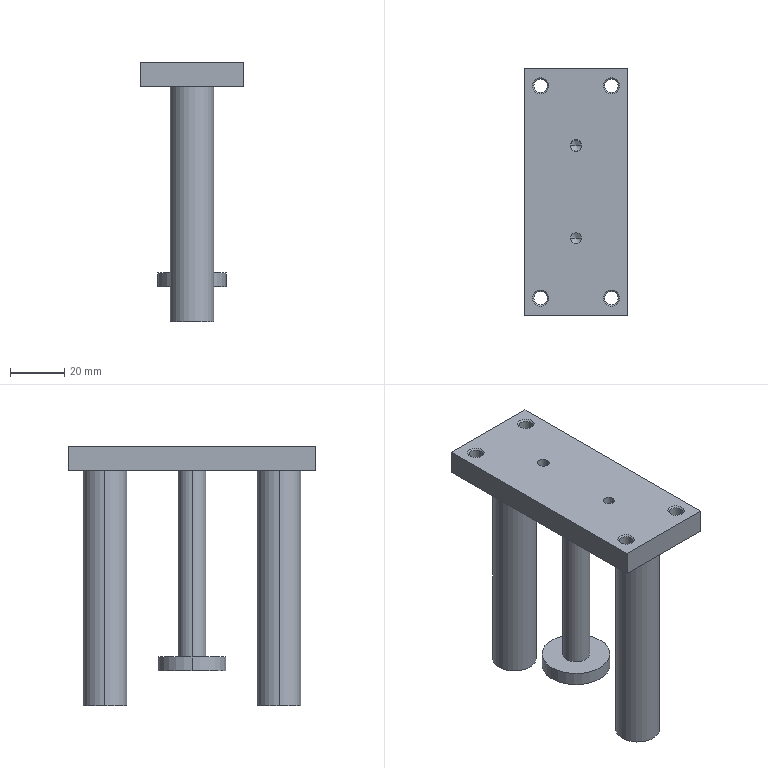Part | SolidWorks | features BaseBody 1 | 1 solid | 56 faces | box 38 x 91 x 95.5 mm | volume 72871 mm3 | cylinder 22 | cone 20 | plane 14 | commonest cylinder face diameters 4.917 x8 4 x6 16 x4 10 x2 25 x2
STEP:
#1=CARTESIAN_POINT('',(-8.,32.,7.));
#2=VERTEX_POINT('',#1);
#3=CARTESIAN_POINT('',(8.,32.,7.));
#4=VERTEX_POINT('',#3);
#5=CARTESIAN_POINT('',(0.,32.,7.));
#6=DIRECTION('',(0.,0.,-1.));
#7=DIRECTION('',(-1.,0.,0.));
#8=AXIS2_PLACEMENT_3D('',#5,#6,#7);
#9=CIRCLE('',#8,8.);
#10=EDGE_CURVE('',#2,#4,#9,.T.);
#11=ORIENTED_EDGE('',*,*,#10,.T.);
#12=CARTESIAN_POINT('',(8.,32.,-79.5));
#13=VERTEX_POINT('',#12);
#14=CARTESIAN_POINT('',(8.,32.,-87.5));
#15=DIRECTION('',(0.,0.,-1.));
#16=VECTOR('',#15,1000.);
#17=LINE('',#14,#16);
#18=EDGE_CURVE('',#4,#13,#17,.T.);
#19=ORIENTED_EDGE('',*,*,#18,.T.);
#20=CARTESIAN_POINT('',(-8.,32.,-79.5));
#21=VERTEX_POINT('',#20);
#22=CARTESIAN_POINT('',(0.,32.,-79.5));
#23=DIRECTION('',(0.,0.,1.));
#24=DIRECTION('',(-1.,0.,0.));
#25=AXIS2_PLACEMENT_3D('',#22,#23,#24);
#26=CIRCLE('',#25,8.);
#27=EDGE_CURVE('',#13,#21,#26,.T.);
#28=ORIENTED_EDGE('',*,*,#27,.T.);
#29=CARTESIAN_POINT('',(-8.,32.,-87.5));
#30=DIRECTION('',(0.,0.,-1.));
#31=VECTOR('',#30,1000.);
#32=LINE('',#29,#31);
#33=EDGE_CURVE('',#2,#21,#32,.T.);
#34=ORIENTED_EDGE('',*,*,#33,.F.);
#35=EDGE_LOOP('',(#11,#19,#28,#34));
#36=FACE_OUTER_BOUND('',#35,.T.);
#37=CARTESIAN_POINT('',(0.,32.,-87.5));
#38=DIRECTION('',(0.,0.,-1.));
#39=DIRECTION('',(-1.,0.,0.));
#40=AXIS2_PLACEMENT_3D('',#37,#38,#39);
#41=CYLINDRICAL_SURFACE('',#40,8.);
#42=ADVANCED_FACE('',(#36),#41,.T.);
#43=CARTESIAN_POINT('',(-8.,-32.,7.));
#44=VERTEX_POINT('',#43);
#45=CARTESIAN_POINT('',(8.,-32.,7.));
#46=VERTEX_POINT('',#45);
#47=CARTESIAN_POINT('',(0.,-32.,7.));
#48=DIRECTION('',(0.,0.,-1.));
#49=DIRECTION('',(-1.,0.,0.));
#50=AXIS2_PLACEMENT_3D('',#47,#48,#49);
#51=CIRCLE('',#50,8.);
#52=EDGE_CURVE('',#44,#46,#51,.T.);
#53=ORIENTED_EDGE('',*,*,#52,.T.);
#54=CARTESIAN_POINT('',(8.,-32.,-79.5));
#55=VERTEX_POINT('',#54);
#56=CARTESIAN_POINT('',(8.,-32.,-87.5));
#57=DIRECTION('',(0.,0.,-1.));
#58=VECTOR('',#57,1000.);
#59=LINE('',#56,#58);
#60=EDGE_CURVE('',#46,#55,#59,.T.);
#61=ORIENTED_EDGE('',*,*,#60,.T.);
#62=CARTESIAN_POINT('',(-8.,-32.,-79.5));
#63=VERTEX_POINT('',#62);
#64=CARTESIAN_POINT('',(0.,-32.,-79.5));
#65=DIRECTION('',(0.,0.,1.));
#66=DIRECTION('',(-1.,0.,0.));
#67=AXIS2_PLACEMENT_3D('',#64,#65,#66);
#68=CIRCLE('',#67,8.);
#69=EDGE_CURVE('',#55,#63,#68,.T.);
#70=ORIENTED_EDGE('',*,*,#69,.T.);
#71=CARTESIAN_POINT('',(-8.,-32.,-87.5));
#72=DIRECTION('',(0.,0.,-1.));
#73=VECTOR('',#72,1000.);
#74=LINE('',#71,#73);
#75=EDGE_CURVE('',#44,#63,#74,.T.);
#76=ORIENTED_EDGE('',*,*,#75,.F.);
#77=EDGE_LOOP('',(#53,#61,#70,#76));
#78=FACE_OUTER_BOUND('',#77,.T.);
#79=CARTESIAN_POINT('',(0.,-32.,-87.5));
#80=DIRECTION('',(0.,0.,-1.));
#81=DIRECTION('',(-1.,0.,0.));
#82=AXIS2_PLACEMENT_3D('',#79,#80,#81);
#83=CYLINDRICAL_SURFACE('',#82,8.);
#84=ADVANCED_FACE('',(#78),#83,.T.);
#85=CARTESIAN_POINT('',(5.,0.,-61.5));
#86=VERTEX_POINT('',#85);
#87=CARTESIAN_POINT('',(-5.,0.,-61.5));
#88=VERTEX_POINT('',#87);
#89=CARTESIAN_POINT('',(0.,0.,-61.5));
#90=DIRECTION('',(0.,0.,1.));
#91=DIRECTION('',(1.,0.,0.));
#92=AXIS2_PLACEMENT_3D('',#89,#90,#91);
#93=CIRCLE('',#92,5.);
#94=EDGE_CURVE('',#86,#88,#93,.T.);
#95=ORIENTED_EDGE('',*,*,#94,.T.);
#96=CARTESIAN_POINT('',(-5.,0.,7.));
#97=VERTEX_POINT('',#96);
#98=CARTESIAN_POINT('',(-5.,0.,-66.5));
#99=DIRECTION('',(0.,0.,1.));
#100=VECTOR('',#99,1000.);
#101=LINE('',#98,#100);
#102=EDGE_CURVE('',#88,#97,#101,.T.);
#103=ORIENTED_EDGE('',*,*,#102,.T.);
#104=CARTESIAN_POINT('',(5.,0.,7.));
#105=VERTEX_POINT('',#104);
#106=CARTESIAN_POINT('',(0.,0.,7.));
#107=DIRECTION('',(0.,0.,-1.));
#108=DIRECTION('',(1.,0.,0.));
#109=AXIS2_PLACEMENT_3D('',#106,#107,#108);
#110=CIRCLE('',#109,5.);
#111=EDGE_CURVE('',#97,#105,#110,.T.);
#112=ORIENTED_EDGE('',*,*,#111,.T.);
#113=CARTESIAN_POINT('',(5.,0.,-66.5));
#114=DIRECTION('',(0.,0.,1.));
#115=VECTOR('',#114,1000.);
#116=LINE('',#113,#115);
#117=EDGE_CURVE('',#86,#105,#116,.T.);
#118=ORIENTED_EDGE('',*,*,#117,.F.);
#119=EDGE_LOOP('',(#95,#103,#112,#118));
#120=FACE_OUTER_BOUND('',#119,.T.);
#121=CARTESIAN_POINT('',(0.,0.,-66.5));
#122=DIRECTION('',(0.,0.,1.));
#123=DIRECTION('',(1.,0.,0.));
#124=AXIS2_PLACEMENT_3D('',#121,#122,#123);
#125=CYLINDRICAL_SURFACE('',#124,5.);
#126=ADVANCED_FACE('',(#120),#125,.T.);
#127=CARTESIAN_POINT('',(15.459,-39.,7.542));
#128=VERTEX_POINT('',#127);
#129=CARTESIAN_POINT('',(10.541,-39.,7.542));
#130=VERTEX_POINT('',#129);
#131=CARTESIAN_POINT('',(13.,-39.,7.542));
#132=DIRECTION('',(0.,0.,-1.));
#133=DIRECTION('',(-1.,0.,0.));
#134=AXIS2_PLACEMENT_3D('',#131,#132,#133);
#135=CIRCLE('',#134,2.459);
#136=EDGE_CURVE('',#128,#130,#135,.T.);
#137=ORIENTED_EDGE('',*,*,#136,.F.);
#138=CARTESIAN_POINT('',(16.,-39.,7.));
#139=VERTEX_POINT('',#138);
#140=CARTESIAN_POINT('',(16.,-39.,7.));
#141=DIRECTION('',(0.7071,0.,-0.7071));
#142=VECTOR('',#141,1000.);
#143=LINE('',#140,#142);
#144=EDGE_CURVE('',#128,#139,#143,.T.);
#145=ORIENTED_EDGE('',*,*,#144,.T.);
#146=CARTESIAN_POINT('',(10.,-39.,7.));
#147=VERTEX_POINT('',#146);
#148=CARTESIAN_POINT('',(13.,-39.,7.));
#149=DIRECTION('',(0.,0.,-1.));
#150=DIRECTION('',(-1.,0.,0.));
#151=AXIS2_PLACEMENT_3D('',#148,#149,#150);
#152=CIRCLE('',#151,3.);
#153=EDGE_CURVE('',#139,#147,#152,.T.);
#154=ORIENTED_EDGE('',*,*,#153,.T.);
#155=CARTESIAN_POINT('',(10.,-39.,7.));
#156=DIRECTION('',(-0.7071,0.,-0.7071));
#157=VECTOR('',#156,1000.);
#158=LINE('',#155,#157);
#159=EDGE_CURVE('',#130,#147,#158,.T.);
#160=ORIENTED_EDGE('',*,*,#159,.F.);
#161=EDGE_LOOP('',(#137,#145,#154,#160));
#162=FACE_OUTER_BOUND('',#161,.T.);
#163=CARTESIAN_POINT('',(13.,-39.,7.));
#164=DIRECTION('',(0.,0.,-1.));
#165=DIRECTION('',(-1.,0.,0.));
#166=AXIS2_PLACEMENT_3D('',#163,#164,#165);
#167=CONICAL_SURFACE('',#166,3.,0.7854);
#168=ADVANCED_FACE('',(#162),#167,.F.);
#169=CARTESIAN_POINT('',(-10.541,-39.,7.542));
#170=VERTEX_POINT('',#169);
#171=CARTESIAN_POINT('',(-15.459,-39.,7.542));
#172=VERTEX_POINT('',#171);
#173=CARTESIAN_POINT('',(-13.,-39.,7.542));
#174=DIRECTION('',(0.,0.,-1.));
#175=DIRECTION('',(-1.,0.,0.));
#176=AXIS2_PLACEMENT_3D('',#173,#174,#175);
#177=CIRCLE('',#176,2.459);
#178=EDGE_CURVE('',#170,#172,#177,.T.);
#179=ORIENTED_EDGE('',*,*,#178,.F.);
#180=CARTESIAN_POINT('',(-10.,-39.,7.));
#181=VERTEX_POINT('',#180);
#182=CARTESIAN_POINT('',(-10.,-39.,7.));
#183=DIRECTION('',(0.7071,0.,-0.7071));
#184=VECTOR('',#183,1000.);
#185=LINE('',#182,#184);
#186=EDGE_CURVE('',#170,#181,#185,.T.);
#187=ORIENTED_EDGE('',*,*,#186,.T.);
#188=CARTESIAN_POINT('',(-16.,-39.,7.));
#189=VERTEX_POINT('',#188);
#190=CARTESIAN_POINT('',(-13.,-39.,7.));
#191=DIRECTION('',(0.,0.,-1.));
#192=DIRECTION('',(-1.,0.,0.));
#193=AXIS2_PLACEMENT_3D('',#190,#191,#192);
#194=CIRCLE('',#193,3.);
#195=EDGE_CURVE('',#181,#189,#194,.T.);
#196=ORIENTED_EDGE('',*,*,#195,.T.);
#197=CARTESIAN_POINT('',(-16.,-39.,7.));
#198=DIRECTION('',(-0.7071,0.,-0.7071));
#199=VECTOR('',#198,1000.);
#200=LINE('',#197,#199);
#201=EDGE_CURVE('',#172,#189,#200,.T.);
#202=ORIENTED_EDGE('',*,*,#201,.F.);
#203=EDGE_LOOP('',(#179,#187,#196,#202));
#204=FACE_OUTER_BOUND('',#203,.T.);
#205=CARTESIAN_POINT('',(-13.,-39.,7.));
#206=DIRECTION('',(0.,0.,-1.));
#207=DIRECTION('',(-1.,0.,0.));
#208=AXIS2_PLACEMENT_3D('',#205,#206,#207);
#209=CONICAL_SURFACE('',#208,3.,0.7854);
#210=ADVANCED_FACE('',(#204),#209,.F.);
#211=CARTESIAN_POINT('',(15.459,39.,7.542));
#212=VERTEX_POINT('',#211);
#213=CARTESIAN_POINT('',(10.541,39.,7.542));
#214=VERTEX_POINT('',#213);
#215=CARTESIAN_POINT('',(13.,39.,7.542));
#216=DIRECTION('',(0.,0.,-1.));
#217=DIRECTION('',(-1.,0.,0.));
#218=AXIS2_PLACEMENT_3D('',#215,#216,#217);
#219=CIRCLE('',#218,2.459);
#220=EDGE_CURVE('',#212,#214,#219,.T.);
#221=ORIENTED_EDGE('',*,*,#220,.F.);
#222=CARTESIAN_POINT('',(16.,39.,7.));
#223=VERTEX_POINT('',#222);
#224=CARTESIAN_POINT('',(16.,39.,7.));
#225=DIRECTION('',(0.7071,0.,-0.7071));
#226=VECTOR('',#225,1000.);
#227=LINE('',#224,#226);
#228=EDGE_CURVE('',#212,#223,#227,.T.);
#229=ORIENTED_EDGE('',*,*,#228,.T.);
#230=CARTESIAN_POINT('',(10.,39.,7.));
#231=VERTEX_POINT('',#230);
#232=CARTESIAN_POINT('',(13.,39.,7.));
#233=DIRECTION('',(0.,0.,-1.));
#234=DIRECTION('',(-1.,0.,0.));
#235=AXIS2_PLACEMENT_3D('',#232,#233,#234);
#236=CIRCLE('',#235,3.);
#237=EDGE_CURVE('',#223,#231,#236,.T.);
#238=ORIENTED_EDGE('',*,*,#237,.T.);
#239=CARTESIAN_POINT('',(10.,39.,7.));
#240=DIRECTION('',(-0.7071,0.,-0.7071));
#241=VECTOR('',#240,1000.);
#242=LINE('',#239,#241);
#243=EDGE_CURVE('',#214,#231,#242,.T.);
#244=ORIENTED_EDGE('',*,*,#243,.F.);
#245=EDGE_LOOP('',(#221,#229,#238,#244));
#246=FACE_OUTER_BOUND('',#245,.T.);
#247=CARTESIAN_POINT('',(13.,39.,7.));
#248=DIRECTION('',(0.,0.,-1.));
#249=DIRECTION('',(-1.,0.,0.));
#250=AXIS2_PLACEMENT_3D('',#247,#248,#249);
#251=CONICAL_SURFACE('',#250,3.,0.7854);
#252=ADVANCED_FACE('',(#246),#251,.F.);
#253=CARTESIAN_POINT('',(-10.541,39.,7.542));
#254=VERTEX_POINT('',#253);
#255=CARTESIAN_POINT('',(-15.459,39.,7.542));
#256=VERTEX_POINT('',#255);
#257=CARTESIAN_POINT('',(-13.,39.,7.542));
#258=DIRECTION('',(0.,0.,-1.));
#259=DIRECTION('',(-1.,0.,0.));
#260=AXIS2_PLACEMENT_3D('',#257,#258,#259);
#261=CIRCLE('',#260,2.459);
#262=EDGE_CURVE('',#254,#256,#261,.T.);
#263=ORIENTED_EDGE('',*,*,#262,.F.);
#264=CARTESIAN_POINT('',(-10.,39.,7.));
#265=VERTEX_POINT('',#264);
#266=CARTESIAN_POINT('',(-10.,39.,7.));
#267=DIRECTION('',(0.7071,0.,-0.7071));
#268=VECTOR('',#267,1000.);
#269=LINE('',#266,#268);
#270=EDGE_CURVE('',#254,#265,#269,.T.);
#271=ORIENTED_EDGE('',*,*,#270,.T.);
#272=CARTESIAN_POINT('',(-16.,39.,7.));
#273=VERTEX_POINT('',#272);
#274=CARTESIAN_POINT('',(-13.,39.,7.));
#275=DIRECTION('',(0.,0.,-1.));
#276=DIRECTION('',(-1.,0.,0.));
#277=AXIS2_PLACEMENT_3D('',#274,#275,#276);
#278=CIRCLE('',#277,3.);
#279=EDGE_CURVE('',#265,#273,#278,.T.);
#280=ORIENTED_EDGE('',*,*,#279,.T.);
#281=CARTESIAN_POINT('',(-16.,39.,7.));
#282=DIRECTION('',(-0.7071,0.,-0.7071));
#283=VECTOR('',#282,1000.);
#284=LINE('',#281,#283);
#285=EDGE_CURVE('',#256,#273,#284,.T.);
#286=ORIENTED_EDGE('',*,*,#285,.F.);
#287=EDGE_LOOP('',(#263,#271,#280,#286));
#288=FACE_OUTER_BOUND('',#287,.T.);
#289=CARTESIAN_POINT('',(-13.,39.,7.));
#290=DIRECTION('',(0.,0.,-1.));
#291=DIRECTION('',(-1.,0.,0.));
#292=AXIS2_PLACEMENT_3D('',#289,#290,#291);
#293=CONICAL_SURFACE('',#292,3.,0.7854);
#294=ADVANCED_FACE('',(#288),#293,.F.);
#295=CARTESIAN_POINT('',(15.459,-39.,15.459));
#296=VERTEX_POINT('',#295);
#297=CARTESIAN_POINT('',(10.542,-39.,15.459));
#298=VERTEX_POINT('',#297);
#299=CARTESIAN_POINT('',(13.,-39.,15.459));
#300=DIRECTION('',(0.,0.,-1.));
#301=DIRECTION('',(-1.,0.,0.));
#302=AXIS2_PLACEMENT_3D('',#299,#300,#301);
#303=CIRCLE('',#302,2.458);
#304=EDGE_CURVE('',#296,#298,#303,.T.);
#305=ORIENTED_EDGE('',*,*,#304,.F.);
#306=CARTESIAN_POINT('',(15.459,-39.,16.));
#307=DIRECTION('',(0.,0.,-1.));
#308=VECTOR('',#307,1000.);
#309=LINE('',#306,#308);
#310=EDGE_CURVE('',#296,#128,#309,.T.);
#311=ORIENTED_EDGE('',*,*,#310,.T.);
#312=ORIENTED_EDGE('',*,*,#136,.T.);
#313=CARTESIAN_POINT('',(10.542,-39.,16.));
#314=DIRECTION('',(0.,0.,-1.));
#315=VECTOR('',#314,1000.);
#316=LINE('',#313,#315);
#317=EDGE_CURVE('',#298,#130,#316,.T.);
#318=ORIENTED_EDGE('',*,*,#317,.F.);
#319=EDGE_LOOP('',(#305,#311,#312,#318));
#320=FACE_OUTER_BOUND('',#319,.T.);
#321=CARTESIAN_POINT('',(13.,-39.,16.));
#322=DIRECTION('',(0.,0.,-1.));
#323=DIRECTION('',(-1.,0.,0.));
#324=AXIS2_PLACEMENT_3D('',#321,#322,#323);
#325=CYLINDRICAL_SURFACE('',#324,2.458);
#326=ADVANCED_FACE('',(#320),#325,.F.);
#327=CARTESIAN_POINT('',(-10.542,-39.,15.459));
#328=VERTEX_POINT('',#327);
#329=CARTESIAN_POINT('',(-15.459,-39.,15.459));
#330=VERTEX_POINT('',#329);
#331=CARTESIAN_POINT('',(-13.,-39.,15.459));
#332=DIRECTION('',(0.,0.,-1.));
#333=DIRECTION('',(-1.,0.,0.));
#334=AXIS2_PLACEMENT_3D('',#331,#332,#333);
#335=CIRCLE('',#334,2.458);
#336=EDGE_CURVE('',#328,#330,#335,.T.);
#337=ORIENTED_EDGE('',*,*,#336,.F.);
#338=CARTESIAN_POINT('',(-10.542,-39.,16.));
#339=DIRECTION('',(0.,0.,-1.));
#340=VECTOR('',#339,1000.);
#341=LINE('',#338,#340);
#342=EDGE_CURVE('',#328,#170,#341,.T.);
#343=ORIENTED_EDGE('',*,*,#342,.T.);
#344=ORIENTED_EDGE('',*,*,#178,.T.);
#345=CARTESIAN_POINT('',(-15.459,-39.,16.));
#346=DIRECTION('',(0.,0.,-1.));
#347=VECTOR('',#346,1000.);
#348=LINE('',#345,#347);
#349=EDGE_CURVE('',#330,#172,#348,.T.);
#350=ORIENTED_EDGE('',*,*,#349,.F.);
#351=EDGE_LOOP('',(#337,#343,#344,#350));
#352=FACE_OUTER_BOUND('',#351,.T.);
#353=CARTESIAN_POINT('',(-13.,-39.,16.));
#354=DIRECTION('',(0.,0.,-1.));
#355=DIRECTION('',(-1.,0.,0.));
#356=AXIS2_PLACEMENT_3D('',#353,#354,#355);
#357=CYLINDRICAL_SURFACE('',#356,2.458);
#358=ADVANCED_FACE('',(#352),#357,.F.);
#359=CARTESIAN_POINT('',(15.459,39.,15.459));
#360=VERTEX_POINT('',#359);
#361=CARTESIAN_POINT('',(10.542,39.,15.459));
#362=VERTEX_POINT('',#361);
#363=CARTESIAN_POINT('',(13.,39.,15.459));
#364=DIRECTION('',(0.,0.,-1.));
#365=DIRECTION('',(-1.,0.,0.));
#366=AXIS2_PLACEMENT_3D('',#363,#364,#365);
#367=CIRCLE('',#366,2.458);
#368=EDGE_CURVE('',#360,#362,#367,.T.);
#369=ORIENTED_EDGE('',*,*,#368,.F.);
#370=CARTESIAN_POINT('',(15.459,39.,16.));
#371=DIRECTION('',(0.,0.,-1.));
#372=VECTOR('',#371,1000.);
#373=LINE('',#370,#372);
#374=EDGE_CURVE('',#360,#212,#373,.T.);
#375=ORIENTED_EDGE('',*,*,#374,.T.);
#376=ORIENTED_EDGE('',*,*,#220,.T.);
#377=CARTESIAN_POINT('',(10.542,39.,16.));
#378=DIRECTION('',(0.,0.,-1.));
#379=VECTOR('',#378,1000.);
#380=LINE('',#377,#379);
#381=EDGE_CURVE('',#362,#214,#380,.T.);
#382=ORIENTED_EDGE('',*,*,#381,.F.);
#383=EDGE_LOOP('',(#369,#375,#376,#382));
#384=FACE_OUTER_BOUND('',#383,.T.);
#385=CARTESIAN_POINT('',(13.,39.,16.));
#386=DIRECTION('',(0.,0.,-1.));
#387=DIRECTION('',(-1.,0.,0.));
#388=AXIS2_PLACEMENT_3D('',#385,#386,#387);
#389=CYLINDRICAL_SURFACE('',#388,2.458);
#390=ADVANCED_FACE('',(#384),#389,.F.);
#391=CARTESIAN_POINT('',(-10.542,39.,15.459));
#392=VERTEX_POINT('',#391);
#393=CARTESIAN_POINT('',(-15.459,39.,15.459));
#394=VERTEX_POINT('',#393);
#395=CARTESIAN_POINT('',(-13.,39.,15.459));
#396=DIRECTION('',(0.,0.,-1.));
#397=DIRECTION('',(-1.,0.,0.));
#398=AXIS2_PLACEMENT_3D('',#395,#396,#397);
#399=CIRCLE('',#398,2.458);
#400=EDGE_CURVE('',#392,#394,#399,.T.);
#401=ORIENTED_EDGE('',*,*,#400,.F.);
#402=CARTESIAN_POINT('',(-10.542,39.,16.));
#403=DIRECTION('',(0.,0.,-1.));
#404=VECTOR('',#403,1000.);
#405=LINE('',#402,#404);
#406=EDGE_CURVE('',#392,#254,#405,.T.);
#407=ORIENTED_EDGE('',*,*,#406,.T.);
#408=ORIENTED_EDGE('',*,*,#262,.T.);
#409=CARTESIAN_POINT('',(-15.459,39.,16.));
#410=DIRECTION('',(0.,0.,-1.));
#411=VECTOR('',#410,1000.);
#412=LINE('',#409,#411);
#413=EDGE_CURVE('',#394,#256,#412,.T.);
#414=ORIENTED_EDGE('',*,*,#413,.F.);
#415=EDGE_LOOP('',(#401,#407,#408,#414));
#416=FACE_OUTER_BOUND('',#415,.T.);
#417=CARTESIAN_POINT('',(-13.,39.,16.));
#418=DIRECTION('',(0.,0.,-1.));
#419=DIRECTION('',(-1.,0.,0.));
#420=AXIS2_PLACEMENT_3D('',#417,#418,#419);
#421=CYLINDRICAL_SURFACE('',#420,2.458);
#422=ADVANCED_FACE('',(#416),#421,.F.);
#423=CARTESIAN_POINT('',(2.,-17.,16.));
#424=VERTEX_POINT('',#423);
#425=CARTESIAN_POINT('',(-2.,-17.,16.));
#426=VERTEX_POINT('',#425);
#427=CARTESIAN_POINT('',(0.,-17.,16.));
#428=DIRECTION('',(0.,0.,-1.));
#429=DIRECTION('',(-1.,0.,0.));
#430=AXIS2_PLACEMENT_3D('',#427,#428,#429);
#431=CIRCLE('',#430,2.);
#432=EDGE_CURVE('',#424,#426,#431,.T.);
#433=ORIENTED_EDGE('',*,*,#432,.F.);
#434=CARTESIAN_POINT('',(2.,-17.,10.));
#435=VERTEX_POINT('',#434);
#436=CARTESIAN_POINT('',(2.,-17.,16.));
#437=DIRECTION('',(0.,0.,-1.));
#438=VECTOR('',#437,1000.);
#439=LINE('',#436,#438);
#440=EDGE_CURVE('',#424,#435,#439,.T.);
#441=ORIENTED_EDGE('',*,*,#440,.T.);
#442=CARTESIAN_POINT('',(-2.,-17.,10.));
#443=VERTEX_POINT('',#442);
#444=CARTESIAN_POINT('',(0.,-17.,10.));
#445=DIRECTION('',(0.,0.,1.));
#446=DIRECTION('',(-1.,0.,0.));
#447=AXIS2_PLACEMENT_3D('',#444,#445,#446);
#448=CIRCLE('',#447,2.);
#449=EDGE_CURVE('',#443,#435,#448,.T.);
#450=ORIENTED_EDGE('',*,*,#449,.F.);
#451=CARTESIAN_POINT('',(-2.,-17.,16.));
#452=DIRECTION('',(0.,0.,-1.));
#453=VECTOR('',#452,1000.);
#454=LINE('',#451,#453);
#455=EDGE_CURVE('',#426,#443,#454,.T.);
#456=ORIENTED_EDGE('',*,*,#455,.F.);
#457=EDGE_LOOP('',(#433,#441,#450,#456));
#458=FACE_OUTER_BOUND('',#457,.T.);
#459=CARTESIAN_POINT('',(0.,-17.,16.));
#460=DIRECTION('',(0.,0.,-1.));
#461=DIRECTION('',(-1.,0.,0.));
#462=AXIS2_PLACEMENT_3D('',#459,#460,#461);
#463=CYLINDRICAL_SURFACE('',#462,2.);
#464=ADVANCED_FACE('',(#458),#463,.F.);
#465=ORIENTED_EDGE('',*,*,#304,.T.);
#466=CARTESIAN_POINT('',(10.,-39.,16.));
#467=VERTEX_POINT('',#466);
#468=CARTESIAN_POINT('',(10.,-39.,16.));
#469=DIRECTION('',(-0.7071,0.,0.7071));
#470=VECTOR('',#469,1000.);
#471=LINE('',#468,#470);
#472=EDGE_CURVE('',#298,#467,#471,.T.);
#473=ORIENTED_EDGE('',*,*,#472,.T.);
#474=CARTESIAN_POINT('',(16.,-39.,16.));
#475=VERTEX_POINT('',#474);
#476=CARTESIAN_POINT('',(13.,-39.,16.));
#477=DIRECTION('',(0.,0.,-1.));
#478=DIRECTION('',(1.,0.,0.));
#479=AXIS2_PLACEMENT_3D('',#476,#477,#478);
#480=CIRCLE('',#479,3.);
#481=EDGE_CURVE('',#475,#467,#480,.T.);
#482=ORIENTED_EDGE('',*,*,#481,.F.);
#483=CARTESIAN_POINT('',(16.,-39.,16.));
#484=DIRECTION('',(0.7071,0.,0.7071));
#485=VECTOR('',#484,1000.);
#486=LINE('',#483,#485);
#487=EDGE_CURVE('',#296,#475,#486,.T.);
#488=ORIENTED_EDGE('',*,*,#487,.F.);
#489=EDGE_LOOP('',(#465,#473,#482,#488));
#490=FACE_OUTER_BOUND('',#489,.T.);
#491=CARTESIAN_POINT('',(13.,-39.,16.));
#492=DIRECTION('',(0.,0.,1.));
#493=DIRECTION('',(1.,0.,0.));
#494=AXIS2_PLACEMENT_3D('',#491,#492,#493);
#495=CONICAL_SURFACE('',#494,3.,0.7854);
#496=ADVANCED_FACE('',(#490),#495,.F.);
#497=ORIENTED_EDGE('',*,*,#336,.T.);
#498=CARTESIAN_POINT('',(-16.,-39.,16.));
#499=VERTEX_POINT('',#498);
#500=CARTESIAN_POINT('',(-16.,-39.,16.));
#501=DIRECTION('',(-0.7071,0.,0.7071));
#502=VECTOR('',#501,1000.);
#503=LINE('',#500,#502);
#504=EDGE_CURVE('',#330,#499,#503,.T.);
#505=ORIENTED_EDGE('',*,*,#504,.T.);
#506=CARTESIAN_POINT('',(-10.,-39.,16.));
#507=VERTEX_POINT('',#506);
#508=CARTESIAN_POINT('',(-13.,-39.,16.));
#509=DIRECTION('',(0.,0.,-1.));
#510=DIRECTION('',(1.,0.,0.));
#511=AXIS2_PLACEMENT_3D('',#508,#509,#510);
#512=CIRCLE('',#511,3.);
#513=EDGE_CURVE('',#507,#499,#512,.T.);
#514=ORIENTED_EDGE('',*,*,#513,.F.);
#515=CARTESIAN_POINT('',(-10.,-39.,16.));
#516=DIRECTION('',(0.7071,0.,0.7071));
#517=VECTOR('',#516,1000.);
#518=LINE('',#515,#517);
#519=EDGE_CURVE('',#328,#507,#518,.T.);
#520=ORIENTED_EDGE('',*,*,#519,.F.);
#521=EDGE_LOOP('',(#497,#505,#514,#520));
#522=FACE_OUTER_BOUND('',#521,.T.);
#523=CARTESIAN_POINT('',(-13.,-39.,16.));
#524=DIRECTION('',(0.,0.,1.));
#525=DIRECTION('',(1.,0.,0.));
#526=AXIS2_PLACEMENT_3D('',#523,#524,#525);
#527=CONICAL_SURFACE('',#526,3.,0.7854);
#528=ADVANCED_FACE('',(#522),#527,.F.);
#529=ORIENTED_EDGE('',*,*,#368,.T.);
#530=CARTESIAN_POINT('',(10.,39.,16.));
#531=VERTEX_POINT('',#530);
#532=CARTESIAN_POINT('',(10.,39.,16.));
#533=DIRECTION('',(-0.7071,0.,0.7071));
#534=VECTOR('',#533,1000.);
#535=LINE('',#532,#534);
#536=EDGE_CURVE('',#362,#531,#535,.T.);
#537=ORIENTED_EDGE('',*,*,#536,.T.);
#538=CARTESIAN_POINT('',(16.,39.,16.));
#539=VERTEX_POINT('',#538);
#540=CARTESIAN_POINT('',(13.,39.,16.));
#541=DIRECTION('',(0.,0.,-1.));
#542=DIRECTION('',(1.,0.,0.));
#543=AXIS2_PLACEMENT_3D('',#540,#541,#542);
#544=CIRCLE('',#543,3.);
#545=EDGE_CURVE('',#539,#531,#544,.T.);
#546=ORIENTED_EDGE('',*,*,#545,.F.);
#547=CARTESIAN_POINT('',(16.,39.,16.));
#548=DIRECTION('',(0.7071,0.,0.7071));
#549=VECTOR('',#548,1000.);
#550=LINE('',#547,#549);
#551=EDGE_CURVE('',#360,#539,#550,.T.);
#552=ORIENTED_EDGE('',*,*,#551,.F.);
#553=EDGE_LOOP('',(#529,#537,#546,#552));
#554=FACE_OUTER_BOUND('',#553,.T.);
#555=CARTESIAN_POINT('',(13.,39.,16.));
#556=DIRECTION('',(0.,0.,1.));
#557=DIRECTION('',(1.,0.,0.));
#558=AXIS2_PLACEMENT_3D('',#555,#556,#557);
#559=CONICAL_SURFACE('',#558,3.,0.7854);
#560=ADVANCED_FACE('',(#554),#559,.F.);
#561=ORIENTED_EDGE('',*,*,#400,.T.);
#562=CARTESIAN_POINT('',(-16.,39.,16.));
#563=VERTEX_POINT('',#562);
#564=CARTESIAN_POINT('',(-16.,39.,16.));
#565=DIRECTION('',(-0.7071,0.,0.7071));
#566=VECTOR('',#565,1000.);
#567=LINE('',#564,#566);
#568=EDGE_CURVE('',#394,#563,#567,.T.);
#569=ORIENTED_EDGE('',*,*,#568,.T.);
#570=CARTESIAN_POINT('',(-10.,39.,16.));
#571=VERTEX_POINT('',#570);
#572=CARTESIAN_POINT('',(-13.,39.,16.));
#573=DIRECTION('',(0.,0.,-1.));
#574=DIRECTION('',(1.,0.,0.));
#575=AXIS2_PLACEMENT_3D('',#572,#573,#574);
#576=CIRCLE('',#575,3.);
#577=EDGE_CURVE('',#571,#563,#576,.T.);
#578=ORIENTED_EDGE('',*,*,#577,.F.);
#579=CARTESIAN_POINT('',(-10.,39.,16.));
#580=DIRECTION('',(0.7071,0.,0.7071));
#581=VECTOR('',#580,1000.);
#582=LINE('',#579,#581);
#583=EDGE_CURVE('',#392,#571,#582,.T.);
#584=ORIENTED_EDGE('',*,*,#583,.F.);
#585=EDGE_LOOP('',(#561,#569,#578,#584));
#586=FACE_OUTER_BOUND('',#585,.T.);
#587=CARTESIAN_POINT('',(-13.,39.,16.));
#588=DIRECTION('',(0.,0.,1.));
#589=DIRECTION('',(1.,0.,0.));
#590=AXIS2_PLACEMENT_3D('',#587,#588,#589);
#591=CONICAL_SURFACE('',#590,3.,0.7854);
#592=ADVANCED_FACE('',(#586),#591,.F.);
#593=CARTESIAN_POINT('',(12.5,0.,-66.5));
#594=VERTEX_POINT('',#593);
#595=CARTESIAN_POINT('',(-12.5,0.,-66.5));
#596=VERTEX_POINT('',#595);
#597=CARTESIAN_POINT('',(0.,0.,-66.5));
#598=DIRECTION('',(0.,0.,1.));
#599=DIRECTION('',(1.,0.,0.));
#600=AXIS2_PLACEMENT_3D('',#597,#598,#599);
#601=CIRCLE('',#600,12.5);
#602=EDGE_CURVE('',#594,#596,#601,.T.);
#603=ORIENTED_EDGE('',*,*,#602,.T.);
#604=CARTESIAN_POINT('',(-12.5,0.,-61.5));
#605=VERTEX_POINT('',#604);
#606=CARTESIAN_POINT('',(-12.5,0.,-66.5));
#607=DIRECTION('',(0.,0.,1.));
#608=VECTOR('',#607,1000.);
#609=LINE('',#606,#608);
#610=EDGE_CURVE('',#596,#605,#609,.T.);
#611=ORIENTED_EDGE('',*,*,#610,.T.);
#612=CARTESIAN_POINT('',(12.5,0.,-61.5));
#613=VERTEX_POINT('',#612);
#614=CARTESIAN_POINT('',(0.,0.,-61.5));
#615=DIRECTION('',(0.,0.,-1.));
#616=DIRECTION('',(1.,0.,0.));
#617=AXIS2_PLACEMENT_3D('',#614,#615,#616);
#618=CIRCLE('',#617,12.5);
#619=EDGE_CURVE('',#605,#613,#618,.T.);
#620=ORIENTED_EDGE('',*,*,#619,.T.);
#621=CARTESIAN_POINT('',(12.5,0.,-66.5));
#622=DIRECTION('',(0.,0.,1.));
#623=VECTOR('',#622,1000.);
#624=LINE('',#621,#623);
#625=EDGE_CURVE('',#594,#613,#624,.T.);
#626=ORIENTED_EDGE('',*,*,#625,.F.);
#627=EDGE_LOOP('',(#603,#611,#620,#626));
#628=FACE_OUTER_BOUND('',#627,.T.);
#629=CARTESIAN_POINT('',(0.,0.,-66.5));
#630=DIRECTION('',(0.,0.,1.));
#631=DIRECTION('',(1.,0.,0.));
#632=AXIS2_PLACEMENT_3D('',#629,#630,#631);
#633=CYLINDRICAL_SURFACE('',#632,12.5);
#634=ADVANCED_FACE('',(#628),#633,.T.);
#635=CARTESIAN_POINT('',(0.,-17.,8.845));
#636=VERTEX_POINT('',#635);
#637=CARTESIAN_POINT('',(2.,-17.,10.));
#638=DIRECTION('',(0.866,0.,0.5));
#639=VECTOR('',#638,1000.);
#640=LINE('',#637,#639);
#641=EDGE_CURVE('',#636,#435,#640,.T.);
#642=ORIENTED_EDGE('',*,*,#641,.F.);
#643=CARTESIAN_POINT('',(-2.,-17.,10.));
#644=DIRECTION('',(-0.866,0.,0.5));
#645=VECTOR('',#644,1000.);
#646=LINE('',#643,#645);
#647=EDGE_CURVE('',#636,#443,#646,.T.);
#648=ORIENTED_EDGE('',*,*,#647,.T.);
#649=ORIENTED_EDGE('',*,*,#449,.T.);
#650=EDGE_LOOP('',(#642,#648,#649));
#651=FACE_OUTER_BOUND('',#650,.T.);
#652=CARTESIAN_POINT('',(0.,-17.,10.));
#653=DIRECTION('',(0.,0.,1.));
#654=DIRECTION('',(1.,0.,0.));
#655=AXIS2_PLACEMENT_3D('',#652,#653,#654);
#656=CONICAL_SURFACE('',#655,2.,1.047);
#657=ADVANCED_FACE('',(#651),#656,.F.);
#658=CARTESIAN_POINT('',(2.,17.,13.));
#659=VERTEX_POINT('',#658);
#660=CARTESIAN_POINT('',(-2.,17.,13.));
#661=VERTEX_POINT('',#660);
#662=CARTESIAN_POINT('',(0.,17.,13.));
#663=DIRECTION('',(0.,0.,-1.));
#664=DIRECTION('',(-1.,0.,0.));
#665=AXIS2_PLACEMENT_3D('',#662,#663,#664);
#666=CIRCLE('',#665,2.);
#667=EDGE_CURVE('',#659,#661,#666,.T.);
#668=ORIENTED_EDGE('',*,*,#667,.F.);
#669=CARTESIAN_POINT('',(2.,17.,10.));
#670=VERTEX_POINT('',#669);
#671=CARTESIAN_POINT('',(2.,17.,16.));
#672=DIRECTION('',(0.,0.,-1.));
#673=VECTOR('',#672,1000.);
#674=LINE('',#671,#673);
#675=EDGE_CURVE('',#659,#670,#674,.T.);
#676=ORIENTED_EDGE('',*,*,#675,.T.);
#677=CARTESIAN_POINT('',(-2.,17.,10.));
#678=VERTEX_POINT('',#677);
#679=CARTESIAN_POINT('',(0.,17.,10.));
#680=DIRECTION('',(0.,0.,1.));
#681=DIRECTION('',(-1.,0.,0.));
#682=AXIS2_PLACEMENT_3D('',#679,#680,#681);
#683=CIRCLE('',#682,2.);
#684=EDGE_CURVE('',#678,#670,#683,.T.);
#685=ORIENTED_EDGE('',*,*,#684,.F.);
#686=CARTESIAN_POINT('',(-2.,17.,16.));
#687=DIRECTION('',(0.,0.,-1.));
#688=VECTOR('',#687,1000.);
#689=LINE('',#686,#688);
#690=EDGE_CURVE('',#661,#678,#689,.T.);
#691=ORIENTED_EDGE('',*,*,#690,.F.);
#692=EDGE_LOOP('',(#668,#676,#685,#691));
#693=FACE_OUTER_BOUND('',#692,.T.);
#694=CARTESIAN_POINT('',(0.,17.,16.));
#695=DIRECTION('',(0.,0.,-1.));
#696=DIRECTION('',(-1.,0.,0.));
#697=AXIS2_PLACEMENT_3D('',#694,#695,#696);
#698=CYLINDRICAL_SURFACE('',#697,2.);
#699=ADVANCED_FACE('',(#693),#698,.F.);
#700=CARTESIAN_POINT('',(0.,17.,8.845));
#701=VERTEX_POINT('',#700);
#702=CARTESIAN_POINT('',(2.,17.,10.));
#703=DIRECTION('',(0.866,0.,0.5));
#704=VECTOR('',#703,1000.);
#705=LINE('',#702,#704);
#706=EDGE_CURVE('',#701,#670,#705,.T.);
#707=ORIENTED_EDGE('',*,*,#706,.F.);
#708=CARTESIAN_POINT('',(-2.,17.,10.));
#709=DIRECTION('',(-0.866,0.,0.5));
#710=VECTOR('',#709,1000.);
#711=LINE('',#708,#710);
#712=EDGE_CURVE('',#701,#678,#711,.T.);
#713=ORIENTED_EDGE('',*,*,#712,.T.);
#714=ORIENTED_EDGE('',*,*,#684,.T.);
#715=EDGE_LOOP('',(#707,#713,#714));
#716=FACE_OUTER_BOUND('',#715,.T.);
#717=CARTESIAN_POINT('',(0.,17.,10.));
#718=DIRECTION('',(0.,0.,1.));
#719=DIRECTION('',(1.,0.,0.));
#720=AXIS2_PLACEMENT_3D('',#717,#718,#719);
#721=CONICAL_SURFACE('',#720,2.,1.047);
#722=ADVANCED_FACE('',(#716),#721,.F.);
#723=ORIENTED_EDGE('',*,*,#18,.F.);
#724=CARTESIAN_POINT('',(0.,32.,7.));
#725=DIRECTION('',(0.,0.,-1.));
#726=DIRECTION('',(-1.,0.,0.));
#727=AXIS2_PLACEMENT_3D('',#724,#725,#726);
#728=CIRCLE('',#727,8.);
#729=EDGE_CURVE('',#4,#2,#728,.T.);
#730=ORIENTED_EDGE('',*,*,#729,.T.);
#731=ORIENTED_EDGE('',*,*,#33,.T.);
#732=CARTESIAN_POINT('',(0.,32.,-79.5));
#733=DIRECTION('',(0.,0.,1.));
#734=DIRECTION('',(-1.,0.,0.));
#735=AXIS2_PLACEMENT_3D('',#732,#733,#734);
#736=CIRCLE('',#735,8.);
#737=EDGE_CURVE('',#21,#13,#736,.T.);
#738=ORIENTED_EDGE('',*,*,#737,.T.);
#739=EDGE_LOOP('',(#723,#730,#731,#738));
#740=FACE_OUTER_BOUND('',#739,.T.);
#741=CARTESIAN_POINT('',(0.,32.,-87.5));
#742=DIRECTION('',(0.,0.,-1.));
#743=DIRECTION('',(-1.,0.,0.));
#744=AXIS2_PLACEMENT_3D('',#741,#742,#743);
#745=CYLINDRICAL_SURFACE('',#744,8.);
#746=ADVANCED_FACE('',(#740),#745,.T.);
#747=ORIENTED_EDGE('',*,*,#737,.F.);
#748=ORIENTED_EDGE('',*,*,#27,.F.);
#749=EDGE_LOOP('',(#747,#748));
#750=FACE_OUTER_BOUND('',#749,.T.);
#751=CARTESIAN_POINT('',(0.,0.,-79.5));
#752=DIRECTION('',(0.,0.,-1.));
#753=DIRECTION('',(-1.,0.,0.));
#754=AXIS2_PLACEMENT_3D('',#751,#752,#753);
#755=PLANE('',#754);
#756=ADVANCED_FACE('',(#750),#755,.T.);
#757=CARTESIAN_POINT('',(19.,45.5,7.));
#758=VERTEX_POINT('',#757);
#759=CARTESIAN_POINT('',(-19.,45.5,7.));
#760=VERTEX_POINT('',#759);
#761=CARTESIAN_POINT('',(0.,45.5,7.));
#762=DIRECTION('',(-1.,0.,0.));
#763=VECTOR('',#762,1000.);
#764=LINE('',#761,#763);
#765=EDGE_CURVE('',#758,#760,#764,.T.);
#766=ORIENTED_EDGE('',*,*,#765,.F.);
#767=CARTESIAN_POINT('',(19.,-45.5,7.));
#768=VERTEX_POINT('',#767);
#769=CARTESIAN_POINT('',(19.,0.,7.));
#770=DIRECTION('',(0.,1.,0.));
#771=VECTOR('',#770,1000.);
#772=LINE('',#769,#771);
#773=EDGE_CURVE('',#768,#758,#772,.T.);
#774=ORIENTED_EDGE('',*,*,#773,.F.);
#775=CARTESIAN_POINT('',(-19.,-45.5,7.));
#776=VERTEX_POINT('',#775);
#777=CARTESIAN_POINT('',(0.,-45.5,7.));
#778=DIRECTION('',(1.,0.,0.));
#779=VECTOR('',#778,1000.);
#780=LINE('',#777,#779);
#781=EDGE_CURVE('',#776,#768,#780,.T.);
#782=ORIENTED_EDGE('',*,*,#781,.F.);
#783=CARTESIAN_POINT('',(-19.,0.,7.));
#784=DIRECTION('',(0.,-1.,0.));
#785=VECTOR('',#784,1000.);
#786=LINE('',#783,#785);
#787=EDGE_CURVE('',#760,#776,#786,.T.);
#788=ORIENTED_EDGE('',*,*,#787,.F.);
#789=EDGE_LOOP('',(#766,#774,#782,#788));
#790=FACE_OUTER_BOUND('',#789,.T.);
#791=ORIENTED_EDGE('',*,*,#10,.F.);
#792=ORIENTED_EDGE('',*,*,#729,.F.);
#793=EDGE_LOOP('',(#791,#792));
#794=FACE_BOUND('',#793,.T.);
#795=ORIENTED_EDGE('',*,*,#52,.F.);
#796=CARTESIAN_POINT('',(0.,-32.,7.));
#797=DIRECTION('',(0.,0.,-1.));
#798=DIRECTION('',(-1.,0.,0.));
#799=AXIS2_PLACEMENT_3D('',#796,#797,#798);
#800=CIRCLE('',#799,8.);
#801=EDGE_CURVE('',#46,#44,#800,.T.);
#802=ORIENTED_EDGE('',*,*,#801,.F.);
#803=EDGE_LOOP('',(#795,#802));
#804=FACE_BOUND('',#803,.T.);
#805=CARTESIAN_POINT('',(0.,0.,7.));
#806=DIRECTION('',(0.,0.,-1.));
#807=DIRECTION('',(1.,0.,0.));
#808=AXIS2_PLACEMENT_3D('',#805,#806,#807);
#809=CIRCLE('',#808,5.);
#810=EDGE_CURVE('',#105,#97,#809,.T.);
#811=ORIENTED_EDGE('',*,*,#810,.F.);
#812=ORIENTED_EDGE('',*,*,#111,.F.);
#813=EDGE_LOOP('',(#811,#812));
#814=FACE_BOUND('',#813,.T.);
#815=CARTESIAN_POINT('',(13.,-39.,7.));
#816=DIRECTION('',(0.,0.,-1.));
#817=DIRECTION('',(-1.,0.,0.));
#818=AXIS2_PLACEMENT_3D('',#815,#816,#817);
#819=CIRCLE('',#818,3.);
#820=EDGE_CURVE('',#147,#139,#819,.T.);
#821=ORIENTED_EDGE('',*,*,#820,.F.);
#822=ORIENTED_EDGE('',*,*,#153,.F.);
#823=EDGE_LOOP('',(#821,#822));
#824=FACE_BOUND('',#823,.T.);
#825=CARTESIAN_POINT('',(-13.,-39.,7.));
#826=DIRECTION('',(0.,0.,-1.));
#827=DIRECTION('',(-1.,0.,0.));
#828=AXIS2_PLACEMENT_3D('',#825,#826,#827);
#829=CIRCLE('',#828,3.);
#830=EDGE_CURVE('',#189,#181,#829,.T.);
#831=ORIENTED_EDGE('',*,*,#830,.F.);
#832=ORIENTED_EDGE('',*,*,#195,.F.);
#833=EDGE_LOOP('',(#831,#832));
#834=FACE_BOUND('',#833,.T.);
#835=CARTESIAN_POINT('',(13.,39.,7.));
#836=DIRECTION('',(0.,0.,-1.));
#837=DIRECTION('',(-1.,0.,0.));
#838=AXIS2_PLACEMENT_3D('',#835,#836,#837);
#839=CIRCLE('',#838,3.);
#840=EDGE_CURVE('',#231,#223,#839,.T.);
#841=ORIENTED_EDGE('',*,*,#840,.F.);
#842=ORIENTED_EDGE('',*,*,#237,.F.);
#843=EDGE_LOOP('',(#841,#842));
#844=FACE_BOUND('',#843,.T.);
#845=CARTESIAN_POINT('',(-13.,39.,7.));
#846=DIRECTION('',(0.,0.,-1.));
#847=DIRECTION('',(-1.,0.,0.));
#848=AXIS2_PLACEMENT_3D('',#845,#846,#847);
#849=CIRCLE('',#848,3.);
#850=EDGE_CURVE('',#273,#265,#849,.T.);
#851=ORIENTED_EDGE('',*,*,#850,.F.);
#852=ORIENTED_EDGE('',*,*,#279,.F.);
#853=EDGE_LOOP('',(#851,#852));
#854=FACE_BOUND('',#853,.T.);
#855=CARTESIAN_POINT('',(0.,0.,7.));
#856=DIRECTION('',(0.,0.,1.));
#857=DIRECTION('',(1.,0.,0.));
#858=AXIS2_PLACEMENT_3D('',#855,#856,#857);
#859=PLANE('',#858);
#860=ADVANCED_FACE('',(#790,#794,#804,#814,#824,#834,#844,#854),#859,.F.);
#861=ORIENTED_EDGE('',*,*,#787,.T.);
#862=CARTESIAN_POINT('',(-19.,-45.5,16.));
#863=VERTEX_POINT('',#862);
#864=CARTESIAN_POINT('',(-19.,-45.5,7.));
#865=DIRECTION('',(0.,0.,1.));
#866=VECTOR('',#865,1000.);
#867=LINE('',#864,#866);
#868=EDGE_CURVE('',#776,#863,#867,.T.);
#869=ORIENTED_EDGE('',*,*,#868,.T.);
#870=CARTESIAN_POINT('',(-19.,45.5,16.));
#871=VERTEX_POINT('',#870);
#872=CARTESIAN_POINT('',(-19.,45.5,16.));
#873=DIRECTION('',(0.,1.,0.));
#874=VECTOR('',#873,1000.);
#875=LINE('',#872,#874);
#876=EDGE_CURVE('',#863,#871,#875,.T.);
#877=ORIENTED_EDGE('',*,*,#876,.T.);
#878=CARTESIAN_POINT('',(-19.,45.5,7.));
#879=DIRECTION('',(0.,0.,-1.));
#880=VECTOR('',#879,1000.);
#881=LINE('',#878,#880);
#882=EDGE_CURVE('',#871,#760,#881,.T.);
#883=ORIENTED_EDGE('',*,*,#882,.T.);
#884=EDGE_LOOP('',(#861,#869,#877,#883));
#885=FACE_OUTER_BOUND('',#884,.T.);
#886=CARTESIAN_POINT('',(-19.,45.5,7.));
#887=DIRECTION('',(-1.,0.,0.));
#888=DIRECTION('',(0.,0.,1.));
#889=AXIS2_PLACEMENT_3D('',#886,#887,#888);
#890=PLANE('',#889);
#891=ADVANCED_FACE('',(#885),#890,.T.);
#892=ORIENTED_EDGE('',*,*,#765,.T.);
#893=ORIENTED_EDGE('',*,*,#882,.F.);
#894=CARTESIAN_POINT('',(19.,45.5,16.));
#895=VERTEX_POINT('',#894);
#896=CARTESIAN_POINT('',(19.,45.5,16.));
#897=DIRECTION('',(1.,0.,0.));
#898=VECTOR('',#897,1000.);
#899=LINE('',#896,#898);
#900=EDGE_CURVE('',#871,#895,#899,.T.);
#901=ORIENTED_EDGE('',*,*,#900,.T.);
#902=CARTESIAN_POINT('',(19.,45.5,7.));
#903=DIRECTION('',(0.,0.,-1.));
#904=VECTOR('',#903,1000.);
#905=LINE('',#902,#904);
#906=EDGE_CURVE('',#895,#758,#905,.T.);
#907=ORIENTED_EDGE('',*,*,#906,.T.);
#908=EDGE_LOOP('',(#892,#893,#901,#907));
#909=FACE_OUTER_BOUND('',#908,.T.);
#910=CARTESIAN_POINT('',(19.,45.5,7.));
#911=DIRECTION('',(0.,1.,0.));
#912=DIRECTION('',(0.,0.,1.));
#913=AXIS2_PLACEMENT_3D('',#910,#911,#912);
#914=PLANE('',#913);
#915=ADVANCED_FACE('',(#909),#914,.T.);
#916=ORIENTED_EDGE('',*,*,#773,.T.);
#917=ORIENTED_EDGE('',*,*,#906,.F.);
#918=CARTESIAN_POINT('',(19.,-45.5,16.));
#919=VERTEX_POINT('',#918);
#920=CARTESIAN_POINT('',(19.,-45.5,16.));
#921=DIRECTION('',(0.,-1.,0.));
#922=VECTOR('',#921,1000.);
#923=LINE('',#920,#922);
#924=EDGE_CURVE('',#895,#919,#923,.T.);
#925=ORIENTED_EDGE('',*,*,#924,.T.);
#926=CARTESIAN_POINT('',(19.,-45.5,7.));
#927=DIRECTION('',(0.,0.,-1.));
#928=VECTOR('',#927,1000.);
#929=LINE('',#926,#928);
#930=EDGE_CURVE('',#919,#768,#929,.T.);
#931=ORIENTED_EDGE('',*,*,#930,.T.);
#932=EDGE_LOOP('',(#916,#917,#925,#931));
#933=FACE_OUTER_BOUND('',#932,.T.);
#934=CARTESIAN_POINT('',(19.,-45.5,7.));
#935=DIRECTION('',(1.,0.,0.));
#936=DIRECTION('',(0.,0.,-1.));
#937=AXIS2_PLACEMENT_3D('',#934,#935,#936);
#938=PLANE('',#937);
#939=ADVANCED_FACE('',(#933),#938,.T.);
#940=ORIENTED_EDGE('',*,*,#781,.T.);
#941=ORIENTED_EDGE('',*,*,#930,.F.);
#942=CARTESIAN_POINT('',(-19.,-45.5,16.));
#943=DIRECTION('',(-1.,0.,0.));
#944=VECTOR('',#943,1000.);
#945=LINE('',#942,#944);
#946=EDGE_CURVE('',#919,#863,#945,.T.);
#947=ORIENTED_EDGE('',*,*,#946,.T.);
#948=ORIENTED_EDGE('',*,*,#868,.F.);
#949=EDGE_LOOP('',(#940,#941,#947,#948));
#950=FACE_OUTER_BOUND('',#949,.T.);
#951=CARTESIAN_POINT('',(-19.,-45.5,7.));
#952=DIRECTION('',(0.,-1.,0.));
#953=DIRECTION('',(0.,0.,-1.));
#954=AXIS2_PLACEMENT_3D('',#951,#952,#953);
#955=PLANE('',#954);
#956=ADVANCED_FACE('',(#950),#955,.T.);
#957=ORIENTED_EDGE('',*,*,#60,.F.);
#958=ORIENTED_EDGE('',*,*,#801,.T.);
#959=ORIENTED_EDGE('',*,*,#75,.T.);
#960=CARTESIAN_POINT('',(0.,-32.,-79.5));
#961=DIRECTION('',(0.,0.,1.));
#962=DIRECTION('',(-1.,0.,0.));
#963=AXIS2_PLACEMENT_3D('',#960,#961,#962);
#964=CIRCLE('',#963,8.);
#965=EDGE_CURVE('',#63,#55,#964,.T.);
#966=ORIENTED_EDGE('',*,*,#965,.T.);
#967=EDGE_LOOP('',(#957,#958,#959,#966));
#968=FACE_OUTER_BOUND('',#967,.T.);
#969=CARTESIAN_POINT('',(0.,-32.,-87.5));
#970=DIRECTION('',(0.,0.,-1.));
#971=DIRECTION('',(-1.,0.,0.));
#972=AXIS2_PLACEMENT_3D('',#969,#970,#971);
#973=CYLINDRICAL_SURFACE('',#972,8.);
#974=ADVANCED_FACE('',(#968),#973,.T.);
#975=ORIENTED_EDGE('',*,*,#102,.F.);
#976=CARTESIAN_POINT('',(0.,0.,-61.5));
#977=DIRECTION('',(0.,0.,1.));
#978=DIRECTION('',(1.,0.,0.));
#979=AXIS2_PLACEMENT_3D('',#976,#977,#978);
#980=CIRCLE('',#979,5.);
#981=EDGE_CURVE('',#88,#86,#980,.T.);
#982=ORIENTED_EDGE('',*,*,#981,.T.);
#983=ORIENTED_EDGE('',*,*,#117,.T.);
#984=ORIENTED_EDGE('',*,*,#810,.T.);
#985=EDGE_LOOP('',(#975,#982,#983,#984));
#986=FACE_OUTER_BOUND('',#985,.T.);
#987=CARTESIAN_POINT('',(0.,0.,-66.5));
#988=DIRECTION('',(0.,0.,1.));
#989=DIRECTION('',(1.,0.,0.));
#990=AXIS2_PLACEMENT_3D('',#987,#988,#989);
#991=CYLINDRICAL_SURFACE('',#990,5.);
#992=ADVANCED_FACE('',(#986),#991,.T.);
#993=ORIENTED_EDGE('',*,*,#144,.F.);
#994=CARTESIAN_POINT('',(13.,-39.,7.542));
#995=DIRECTION('',(0.,0.,-1.));
#996=DIRECTION('',(-1.,0.,0.));
#997=AXIS2_PLACEMENT_3D('',#994,#995,#996);
#998=CIRCLE('',#997,2.459);
#999=EDGE_CURVE('',#130,#128,#998,.T.);
#1000=ORIENTED_EDGE('',*,*,#999,.F.);
#1001=ORIENTED_EDGE('',*,*,#159,.T.);
#1002=ORIENTED_EDGE('',*,*,#820,.T.);
#1003=EDGE_LOOP('',(#993,#1000,#1001,#1002));
#1004=FACE_OUTER_BOUND('',#1003,.T.);
#1005=CARTESIAN_POINT('',(13.,-39.,7.));
#1006=DIRECTION('',(0.,0.,-1.));
#1007=DIRECTION('',(-1.,0.,0.));
#1008=AXIS2_PLACEMENT_3D('',#1005,#1006,#1007);
#1009=CONICAL_SURFACE('',#1008,3.,0.7854);
#1010=ADVANCED_FACE('',(#1004),#1009,.F.);
#1011=ORIENTED_EDGE('',*,*,#186,.F.);
#1012=CARTESIAN_POINT('',(-13.,-39.,7.542));
#1013=DIRECTION('',(0.,0.,-1.));
#1014=DIRECTION('',(-1.,0.,0.));
#1015=AXIS2_PLACEMENT_3D('',#1012,#1013,#1014);
#1016=CIRCLE('',#1015,2.459);
#1017=EDGE_CURVE('',#172,#170,#1016,.T.);
#1018=ORIENTED_EDGE('',*,*,#1017,.F.);
#1019=ORIENTED_EDGE('',*,*,#201,.T.);
#1020=ORIENTED_EDGE('',*,*,#830,.T.);
#1021=EDGE_LOOP('',(#1011,#1018,#1019,#1020));
#1022=FACE_OUTER_BOUND('',#1021,.T.);
#1023=CARTESIAN_POINT('',(-13.,-39.,7.));
#1024=DIRECTION('',(0.,0.,-1.));
#1025=DIRECTION('',(-1.,0.,0.));
#1026=AXIS2_PLACEMENT_3D('',#1023,#1024,#1025);
#1027=CONICAL_SURFACE('',#1026,3.,0.7854);
#1028=ADVANCED_FACE('',(#1022),#1027,.F.);
#1029=ORIENTED_EDGE('',*,*,#228,.F.);
#1030=CARTESIAN_POINT('',(13.,39.,7.542));
#1031=DIRECTION('',(0.,0.,-1.));
#1032=DIRECTION('',(-1.,0.,0.));
#1033=AXIS2_PLACEMENT_3D('',#1030,#1031,#1032);
#1034=CIRCLE('',#1033,2.459);
#1035=EDGE_CURVE('',#214,#212,#1034,.T.);
#1036=ORIENTED_EDGE('',*,*,#1035,.F.);
#1037=ORIENTED_EDGE('',*,*,#243,.T.);
#1038=ORIENTED_EDGE('',*,*,#840,.T.);
#1039=EDGE_LOOP('',(#1029,#1036,#1037,#1038));
#1040=FACE_OUTER_BOUND('',#1039,.T.);
#1041=CARTESIAN_POINT('',(13.,39.,7.));
#1042=DIRECTION('',(0.,0.,-1.));
#1043=DIRECTION('',(-1.,0.,0.));
#1044=AXIS2_PLACEMENT_3D('',#1041,#1042,#1043);
#1045=CONICAL_SURFACE('',#1044,3.,0.7854);
#1046=ADVANCED_FACE('',(#1040),#1045,.F.);
#1047=ORIENTED_EDGE('',*,*,#270,.F.);
#1048=CARTESIAN_POINT('',(-13.,39.,7.542));
#1049=DIRECTION('',(0.,0.,-1.));
#1050=DIRECTION('',(-1.,0.,0.));
#1051=AXIS2_PLACEMENT_3D('',#1048,#1049,#1050);
#1052=CIRCLE('',#1051,2.459);
#1053=EDGE_CURVE('',#256,#254,#1052,.T.);
#1054=ORIENTED_EDGE('',*,*,#1053,.F.);
#1055=ORIENTED_EDGE('',*,*,#285,.T.);
#1056=ORIENTED_EDGE('',*,*,#850,.T.);
#1057=EDGE_LOOP('',(#1047,#1054,#1055,#1056));
#1058=FACE_OUTER_BOUND('',#1057,.T.);
#1059=CARTESIAN_POINT('',(-13.,39.,7.));
#1060=DIRECTION('',(0.,0.,-1.));
#1061=DIRECTION('',(-1.,0.,0.));
#1062=AXIS2_PLACEMENT_3D('',#1059,#1060,#1061);
#1063=CONICAL_SURFACE('',#1062,3.,0.7854);
#1064=ADVANCED_FACE('',(#1058),#1063,.F.);
#1065=ORIENTED_EDGE('',*,*,#924,.F.);
#1066=ORIENTED_EDGE('',*,*,#900,.F.);
#1067=ORIENTED_EDGE('',*,*,#876,.F.);
#1068=ORIENTED_EDGE('',*,*,#946,.F.);
#1069=EDGE_LOOP('',(#1065,#1066,#1067,#1068));
#1070=FACE_OUTER_BOUND('',#1069,.T.);
#1071=CARTESIAN_POINT('',(2.,16.75,16.));
#1072=VERTEX_POINT('',#1071);
#1073=CARTESIAN_POINT('',(-2.,16.75,16.));
#1074=VERTEX_POINT('',#1073);
#1075=CARTESIAN_POINT('',(0.,16.75,16.));
#1076=DIRECTION('',(0.,0.,-1.));
#1077=DIRECTION('',(-1.,0.,0.));
#1078=AXIS2_PLACEMENT_3D('',#1075,#1076,#1077);
#1079=CIRCLE('',#1078,2.);
#1080=EDGE_CURVE('',#1072,#1074,#1079,.T.);
#1081=ORIENTED_EDGE('',*,*,#1080,.T.);
#1082=CARTESIAN_POINT('',(-2.,17.25,16.));
#1083=VERTEX_POINT('',#1082);
#1084=CARTESIAN_POINT('',(-2.,17.25,16.));
#1085=DIRECTION('',(0.,1.,0.));
#1086=VECTOR('',#1085,1000.);
#1087=LINE('',#1084,#1086);
#1088=EDGE_CURVE('',#1074,#1083,#1087,.T.);
#1089=ORIENTED_EDGE('',*,*,#1088,.T.);
#1090=CARTESIAN_POINT('',(2.,17.25,16.));
#1091=VERTEX_POINT('',#1090);
#1092=CARTESIAN_POINT('',(0.,17.25,16.));
#1093=DIRECTION('',(0.,0.,-1.));
#1094=DIRECTION('',(-1.,0.,0.));
#1095=AXIS2_PLACEMENT_3D('',#1092,#1093,#1094);
#1096=CIRCLE('',#1095,2.);
#1097=EDGE_CURVE('',#1083,#1091,#1096,.T.);
#1098=ORIENTED_EDGE('',*,*,#1097,.T.);
#1099=CARTESIAN_POINT('',(2.,16.75,16.));
#1100=DIRECTION('',(0.,-1.,0.));
#1101=VECTOR('',#1100,1000.);
#1102=LINE('',#1099,#1101);
#1103=EDGE_CURVE('',#1091,#1072,#1102,.T.);
#1104=ORIENTED_EDGE('',*,*,#1103,.T.);
#1105=EDGE_LOOP('',(#1081,#1089,#1098,#1104));
#1106=FACE_BOUND('',#1105,.T.);
#1107=CARTESIAN_POINT('',(0.,-17.,16.));
#1108=DIRECTION('',(0.,0.,-1.));
#1109=DIRECTION('',(-1.,0.,0.));
#1110=AXIS2_PLACEMENT_3D('',#1107,#1108,#1109);
#1111=CIRCLE('',#1110,2.);
#1112=EDGE_CURVE('',#426,#424,#1111,.T.);
#1113=ORIENTED_EDGE('',*,*,#1112,.T.);
#1114=ORIENTED_EDGE('',*,*,#432,.T.);
#1115=EDGE_LOOP('',(#1113,#1114));
#1116=FACE_BOUND('',#1115,.T.);
#1117=ORIENTED_EDGE('',*,*,#481,.T.);
#1118=CARTESIAN_POINT('',(13.,-39.,16.));
#1119=DIRECTION('',(0.,0.,-1.));
#1120=DIRECTION('',(1.,0.,0.));
#1121=AXIS2_PLACEMENT_3D('',#1118,#1119,#1120);
#1122=CIRCLE('',#1121,3.);
#1123=EDGE_CURVE('',#467,#475,#1122,.T.);
#1124=ORIENTED_EDGE('',*,*,#1123,.T.);
#1125=EDGE_LOOP('',(#1117,#1124));
#1126=FACE_BOUND('',#1125,.T.);
#1127=ORIENTED_EDGE('',*,*,#513,.T.);
#1128=CARTESIAN_POINT('',(-13.,-39.,16.));
#1129=DIRECTION('',(0.,0.,-1.));
#1130=DIRECTION('',(1.,0.,0.));
#1131=AXIS2_PLACEMENT_3D('',#1128,#1129,#1130);
#1132=CIRCLE('',#1131,3.);
#1133=EDGE_CURVE('',#499,#507,#1132,.T.);
#1134=ORIENTED_EDGE('',*,*,#1133,.T.);
#1135=EDGE_LOOP('',(#1127,#1134));
#1136=FACE_BOUND('',#1135,.T.);
#1137=ORIENTED_EDGE('',*,*,#545,.T.);
#1138=CARTESIAN_POINT('',(13.,39.,16.));
#1139=DIRECTION('',(0.,0.,-1.));
#1140=DIRECTION('',(1.,0.,0.));
#1141=AXIS2_PLACEMENT_3D('',#1138,#1139,#1140);
#1142=CIRCLE('',#1141,3.);
#1143=EDGE_CURVE('',#531,#539,#1142,.T.);
#1144=ORIENTED_EDGE('',*,*,#1143,.T.);
#1145=EDGE_LOOP('',(#1137,#1144));
#1146=FACE_BOUND('',#1145,.T.);
#1147=ORIENTED_EDGE('',*,*,#577,.T.);
#1148=CARTESIAN_POINT('',(-13.,39.,16.));
#1149=DIRECTION('',(0.,0.,-1.));
#1150=DIRECTION('',(1.,0.,0.));
#1151=AXIS2_PLACEMENT_3D('',#1148,#1149,#1150);
#1152=CIRCLE('',#1151,3.);
#1153=EDGE_CURVE('',#563,#571,#1152,.T.);
#1154=ORIENTED_EDGE('',*,*,#1153,.T.);
#1155=EDGE_LOOP('',(#1147,#1154));
#1156=FACE_BOUND('',#1155,.T.);
#1157=CARTESIAN_POINT('',(0.,0.,16.));
#1158=DIRECTION('',(0.,0.,1.));
#1159=DIRECTION('',(1.,0.,0.));
#1160=AXIS2_PLACEMENT_3D('',#1157,#1158,#1159);
#1161=PLANE('',#1160);
#1162=ADVANCED_FACE('',(#1070,#1106,#1116,#1126,#1136,#1146,#1156),#1161,.T.);
#1163=ORIENTED_EDGE('',*,*,#965,.F.);
#1164=ORIENTED_EDGE('',*,*,#69,.F.);
#1165=EDGE_LOOP('',(#1163,#1164));
#1166=FACE_OUTER_BOUND('',#1165,.T.);
#1167=CARTESIAN_POINT('',(0.,0.,-79.5));
#1168=DIRECTION('',(0.,0.,-1.));
#1169=DIRECTION('',(-1.,0.,0.));
#1170=AXIS2_PLACEMENT_3D('',#1167,#1168,#1169);
#1171=PLANE('',#1170);
#1172=ADVANCED_FACE('',(#1166),#1171,.T.);
#1173=ORIENTED_EDGE('',*,*,#94,.F.);
#1174=ORIENTED_EDGE('',*,*,#981,.F.);
#1175=EDGE_LOOP('',(#1173,#1174));
#1176=FACE_BOUND('',#1175,.T.);
#1177=CARTESIAN_POINT('',(0.,0.,-61.5));
#1178=DIRECTION('',(0.,0.,-1.));
#1179=DIRECTION('',(1.,0.,0.));
#1180=AXIS2_PLACEMENT_3D('',#1177,#1178,#1179);
#1181=CIRCLE('',#1180,12.5);
#1182=EDGE_CURVE('',#613,#605,#1181,.T.);
#1183=ORIENTED_EDGE('',*,*,#1182,.F.);
#1184=ORIENTED_EDGE('',*,*,#619,.F.);
#1185=EDGE_LOOP('',(#1183,#1184));
#1186=FACE_OUTER_BOUND('',#1185,.T.);
#1187=CARTESIAN_POINT('',(0.,5.,-61.5));
#1188=DIRECTION('',(0.,0.,-1.));
#1189=DIRECTION('',(-1.,0.,0.));
#1190=AXIS2_PLACEMENT_3D('',#1187,#1188,#1189);
#1191=PLANE('',#1190);
#1192=ADVANCED_FACE('',(#1176,#1186),#1191,.F.);
#1193=ORIENTED_EDGE('',*,*,#310,.F.);
#1194=CARTESIAN_POINT('',(13.,-39.,15.459));
#1195=DIRECTION('',(0.,0.,-1.));
#1196=DIRECTION('',(-1.,0.,0.));
#1197=AXIS2_PLACEMENT_3D('',#1194,#1195,#1196);
#1198=CIRCLE('',#1197,2.458);
#1199=EDGE_CURVE('',#298,#296,#1198,.T.);
#1200=ORIENTED_EDGE('',*,*,#1199,.F.);
#1201=ORIENTED_EDGE('',*,*,#317,.T.);
#1202=ORIENTED_EDGE('',*,*,#999,.T.);
#1203=EDGE_LOOP('',(#1193,#1200,#1201,#1202));
#1204=FACE_OUTER_BOUND('',#1203,.T.);
#1205=CARTESIAN_POINT('',(13.,-39.,16.));
#1206=DIRECTION('',(0.,0.,-1.));
#1207=DIRECTION('',(-1.,0.,0.));
#1208=AXIS2_PLACEMENT_3D('',#1205,#1206,#1207);
#1209=CYLINDRICAL_SURFACE('',#1208,2.458);
#1210=ADVANCED_FACE('',(#1204),#1209,.F.);
#1211=ORIENTED_EDGE('',*,*,#342,.F.);
#1212=CARTESIAN_POINT('',(-13.,-39.,15.459));
#1213=DIRECTION('',(0.,0.,-1.));
#1214=DIRECTION('',(-1.,0.,0.));
#1215=AXIS2_PLACEMENT_3D('',#1212,#1213,#1214);
#1216=CIRCLE('',#1215,2.458);
#1217=EDGE_CURVE('',#330,#328,#1216,.T.);
#1218=ORIENTED_EDGE('',*,*,#1217,.F.);
#1219=ORIENTED_EDGE('',*,*,#349,.T.);
#1220=ORIENTED_EDGE('',*,*,#1017,.T.);
#1221=EDGE_LOOP('',(#1211,#1218,#1219,#1220));
#1222=FACE_OUTER_BOUND('',#1221,.T.);
#1223=CARTESIAN_POINT('',(-13.,-39.,16.));
#1224=DIRECTION('',(0.,0.,-1.));
#1225=DIRECTION('',(-1.,0.,0.));
#1226=AXIS2_PLACEMENT_3D('',#1223,#1224,#1225);
#1227=CYLINDRICAL_SURFACE('',#1226,2.458);
#1228=ADVANCED_FACE('',(#1222),#1227,.F.);
#1229=ORIENTED_EDGE('',*,*,#374,.F.);
#1230=CARTESIAN_POINT('',(13.,39.,15.459));
#1231=DIRECTION('',(0.,0.,-1.));
#1232=DIRECTION('',(-1.,0.,0.));
#1233=AXIS2_PLACEMENT_3D('',#1230,#1231,#1232);
#1234=CIRCLE('',#1233,2.458);
#1235=EDGE_CURVE('',#362,#360,#1234,.T.);
#1236=ORIENTED_EDGE('',*,*,#1235,.F.);
#1237=ORIENTED_EDGE('',*,*,#381,.T.);
#1238=ORIENTED_EDGE('',*,*,#1035,.T.);
#1239=EDGE_LOOP('',(#1229,#1236,#1237,#1238));
#1240=FACE_OUTER_BOUND('',#1239,.T.);
#1241=CARTESIAN_POINT('',(13.,39.,16.));
#1242=DIRECTION('',(0.,0.,-1.));
#1243=DIRECTION('',(-1.,0.,0.));
#1244=AXIS2_PLACEMENT_3D('',#1241,#1242,#1243);
#1245=CYLINDRICAL_SURFACE('',#1244,2.458);
#1246=ADVANCED_FACE('',(#1240),#1245,.F.);
#1247=ORIENTED_EDGE('',*,*,#406,.F.);
#1248=CARTESIAN_POINT('',(-13.,39.,15.459));
#1249=DIRECTION('',(0.,0.,-1.));
#1250=DIRECTION('',(-1.,0.,0.));
#1251=AXIS2_PLACEMENT_3D('',#1248,#1249,#1250);
#1252=CIRCLE('',#1251,2.458);
#1253=EDGE_CURVE('',#394,#392,#1252,.T.);
#1254=ORIENTED_EDGE('',*,*,#1253,.F.);
#1255=ORIENTED_EDGE('',*,*,#413,.T.);
#1256=ORIENTED_EDGE('',*,*,#1053,.T.);
#1257=EDGE_LOOP('',(#1247,#1254,#1255,#1256));
#1258=FACE_OUTER_BOUND('',#1257,.T.);
#1259=CARTESIAN_POINT('',(-13.,39.,16.));
#1260=DIRECTION('',(0.,0.,-1.));
#1261=DIRECTION('',(-1.,0.,0.));
#1262=AXIS2_PLACEMENT_3D('',#1259,#1260,#1261);
#1263=CYLINDRICAL_SURFACE('',#1262,2.458);
#1264=ADVANCED_FACE('',(#1258),#1263,.F.);
#1265=CARTESIAN_POINT('',(2.,16.75,13.));
#1266=VERTEX_POINT('',#1265);
#1267=CARTESIAN_POINT('',(2.,16.75,13.));
#1268=DIRECTION('',(0.,0.,1.));
#1269=VECTOR('',#1268,1000.);
#1270=LINE('',#1267,#1269);
#1271=EDGE_CURVE('',#1266,#1072,#1270,.T.);
#1272=ORIENTED_EDGE('',*,*,#1271,.F.);
#1273=CARTESIAN_POINT('',(-2.,16.75,13.));
#1274=VERTEX_POINT('',#1273);
#1275=CARTESIAN_POINT('',(0.,16.75,13.));
#1276=DIRECTION('',(0.,0.,1.));
#1277=DIRECTION('',(-1.,0.,0.));
#1278=AXIS2_PLACEMENT_3D('',#1275,#1276,#1277);
#1279=CIRCLE('',#1278,2.);
#1280=EDGE_CURVE('',#1274,#1266,#1279,.T.);
#1281=ORIENTED_EDGE('',*,*,#1280,.F.);
#1282=CARTESIAN_POINT('',(-2.,16.75,13.));
#1283=DIRECTION('',(0.,0.,-1.));
#1284=VECTOR('',#1283,1000.);
#1285=LINE('',#1282,#1284);
#1286=EDGE_CURVE('',#1074,#1274,#1285,.T.);
#1287=ORIENTED_EDGE('',*,*,#1286,.F.);
#1288=ORIENTED_EDGE('',*,*,#1080,.F.);
#1289=EDGE_LOOP('',(#1272,#1281,#1287,#1288));
#1290=FACE_OUTER_BOUND('',#1289,.T.);
#1291=CARTESIAN_POINT('',(0.,16.75,13.));
#1292=DIRECTION('',(0.,0.,-1.));
#1293=DIRECTION('',(-1.,0.,0.));
#1294=AXIS2_PLACEMENT_3D('',#1291,#1292,#1293);
#1295=CYLINDRICAL_SURFACE('',#1294,2.);
#1296=ADVANCED_FACE('',(#1290),#1295,.F.);
#1297=CARTESIAN_POINT('',(-2.,17.25,13.));
#1298=VERTEX_POINT('',#1297);
#1299=CARTESIAN_POINT('',(-2.,17.25,13.));
#1300=DIRECTION('',(0.,0.,1.));
#1301=VECTOR('',#1300,1000.);
#1302=LINE('',#1299,#1301);
#1303=EDGE_CURVE('',#1298,#1083,#1302,.T.);
#1304=ORIENTED_EDGE('',*,*,#1303,.F.);
#1305=CARTESIAN_POINT('',(2.,17.25,13.));
#1306=VERTEX_POINT('',#1305);
#1307=CARTESIAN_POINT('',(0.,17.25,13.));
#1308=DIRECTION('',(0.,0.,1.));
#1309=DIRECTION('',(-1.,0.,0.));
#1310=AXIS2_PLACEMENT_3D('',#1307,#1308,#1309);
#1311=CIRCLE('',#1310,2.);
#1312=EDGE_CURVE('',#1306,#1298,#1311,.T.);
#1313=ORIENTED_EDGE('',*,*,#1312,.F.);
#1314=CARTESIAN_POINT('',(2.,17.25,13.));
#1315=DIRECTION('',(0.,0.,-1.));
#1316=VECTOR('',#1315,1000.);
#1317=LINE('',#1314,#1316);
#1318=EDGE_CURVE('',#1091,#1306,#1317,.T.);
#1319=ORIENTED_EDGE('',*,*,#1318,.F.);
#1320=ORIENTED_EDGE('',*,*,#1097,.F.);
#1321=EDGE_LOOP('',(#1304,#1313,#1319,#1320));
#1322=FACE_OUTER_BOUND('',#1321,.T.);
#1323=CARTESIAN_POINT('',(0.,17.25,13.));
#1324=DIRECTION('',(0.,0.,-1.));
#1325=DIRECTION('',(-1.,0.,0.));
#1326=AXIS2_PLACEMENT_3D('',#1323,#1324,#1325);
#1327=CYLINDRICAL_SURFACE('',#1326,2.);
#1328=ADVANCED_FACE('',(#1322),#1327,.F.);
#1329=ORIENTED_EDGE('',*,*,#440,.F.);
#1330=ORIENTED_EDGE('',*,*,#1112,.F.);
#1331=ORIENTED_EDGE('',*,*,#455,.T.);
#1332=CARTESIAN_POINT('',(0.,-17.,10.));
#1333=DIRECTION('',(0.,0.,1.));
#1334=DIRECTION('',(-1.,0.,0.));
#1335=AXIS2_PLACEMENT_3D('',#1332,#1333,#1334);
#1336=CIRCLE('',#1335,2.);
#1337=EDGE_CURVE('',#435,#443,#1336,.T.);
#1338=ORIENTED_EDGE('',*,*,#1337,.F.);
#1339=EDGE_LOOP('',(#1329,#1330,#1331,#1338));
#1340=FACE_OUTER_BOUND('',#1339,.T.);
#1341=CARTESIAN_POINT('',(0.,-17.,16.));
#1342=DIRECTION('',(0.,0.,-1.));
#1343=DIRECTION('',(-1.,0.,0.));
#1344=AXIS2_PLACEMENT_3D('',#1341,#1342,#1343);
#1345=CYLINDRICAL_SURFACE('',#1344,2.);
#1346=ADVANCED_FACE('',(#1340),#1345,.F.);
#1347=ORIENTED_EDGE('',*,*,#472,.F.);
#1348=ORIENTED_EDGE('',*,*,#1199,.T.);
#1349=ORIENTED_EDGE('',*,*,#487,.T.);
#1350=ORIENTED_EDGE('',*,*,#1123,.F.);
#1351=EDGE_LOOP('',(#1347,#1348,#1349,#1350));
#1352=FACE_OUTER_BOUND('',#1351,.T.);
#1353=CARTESIAN_POINT('',(13.,-39.,16.));
#1354=DIRECTION('',(0.,0.,1.));
#1355=DIRECTION('',(1.,0.,0.));
#1356=AXIS2_PLACEMENT_3D('',#1353,#1354,#1355);
#1357=CONICAL_SURFACE('',#1356,3.,0.7854);
#1358=ADVANCED_FACE('',(#1352),#1357,.F.);
#1359=ORIENTED_EDGE('',*,*,#504,.F.);
#1360=ORIENTED_EDGE('',*,*,#1217,.T.);
#1361=ORIENTED_EDGE('',*,*,#519,.T.);
#1362=ORIENTED_EDGE('',*,*,#1133,.F.);
#1363=EDGE_LOOP('',(#1359,#1360,#1361,#1362));
#1364=FACE_OUTER_BOUND('',#1363,.T.);
#1365=CARTESIAN_POINT('',(-13.,-39.,16.));
#1366=DIRECTION('',(0.,0.,1.));
#1367=DIRECTION('',(1.,0.,0.));
#1368=AXIS2_PLACEMENT_3D('',#1365,#1366,#1367);
#1369=CONICAL_SURFACE('',#1368,3.,0.7854);
#1370=ADVANCED_FACE('',(#1364),#1369,.F.);
#1371=ORIENTED_EDGE('',*,*,#536,.F.);
#1372=ORIENTED_EDGE('',*,*,#1235,.T.);
#1373=ORIENTED_EDGE('',*,*,#551,.T.);
#1374=ORIENTED_EDGE('',*,*,#1143,.F.);
#1375=EDGE_LOOP('',(#1371,#1372,#1373,#1374));
#1376=FACE_OUTER_BOUND('',#1375,.T.);
#1377=CARTESIAN_POINT('',(13.,39.,16.));
#1378=DIRECTION('',(0.,0.,1.));
#1379=DIRECTION('',(1.,0.,0.));
#1380=AXIS2_PLACEMENT_3D('',#1377,#1378,#1379);
#1381=CONICAL_SURFACE('',#1380,3.,0.7854);
#1382=ADVANCED_FACE('',(#1376),#1381,.F.);
#1383=ORIENTED_EDGE('',*,*,#568,.F.);
#1384=ORIENTED_EDGE('',*,*,#1253,.T.);
#1385=ORIENTED_EDGE('',*,*,#583,.T.);
#1386=ORIENTED_EDGE('',*,*,#1153,.F.);
#1387=EDGE_LOOP('',(#1383,#1384,#1385,#1386));
#1388=FACE_OUTER_BOUND('',#1387,.T.);
#1389=CARTESIAN_POINT('',(-13.,39.,16.));
#1390=DIRECTION('',(0.,0.,1.));
#1391=DIRECTION('',(1.,0.,0.));
#1392=AXIS2_PLACEMENT_3D('',#1389,#1390,#1391);
#1393=CONICAL_SURFACE('',#1392,3.,0.7854);
#1394=ADVANCED_FACE('',(#1388),#1393,.F.);
#1395=ORIENTED_EDGE('',*,*,#610,.F.);
#1396=CARTESIAN_POINT('',(0.,0.,-66.5));
#1397=DIRECTION('',(0.,0.,1.));
#1398=DIRECTION('',(1.,0.,0.));
#1399=AXIS2_PLACEMENT_3D('',#1396,#1397,#1398);
#1400=CIRCLE('',#1399,12.5);
#1401=EDGE_CURVE('',#596,#594,#1400,.T.);
#1402=ORIENTED_EDGE('',*,*,#1401,.T.);
#1403=ORIENTED_EDGE('',*,*,#625,.T.);
#1404=ORIENTED_EDGE('',*,*,#1182,.T.);
#1405=EDGE_LOOP('',(#1395,#1402,#1403,#1404));
#1406=FACE_OUTER_BOUND('',#1405,.T.);
#1407=CARTESIAN_POINT('',(0.,0.,-66.5));
#1408=DIRECTION('',(0.,0.,1.));
#1409=DIRECTION('',(1.,0.,0.));
#1410=AXIS2_PLACEMENT_3D('',#1407,#1408,#1409);
#1411=CYLINDRICAL_SURFACE('',#1410,12.5);
#1412=ADVANCED_FACE('',(#1406),#1411,.T.);
#1413=ORIENTED_EDGE('',*,*,#1271,.T.);
#1414=ORIENTED_EDGE('',*,*,#1103,.F.);
#1415=ORIENTED_EDGE('',*,*,#1318,.T.);
#1416=CARTESIAN_POINT('',(2.,16.75,13.));
#1417=DIRECTION('',(0.,1.,0.));
#1418=VECTOR('',#1417,1000.);
#1419=LINE('',#1416,#1418);
#1420=EDGE_CURVE('',#659,#1306,#1419,.T.);
#1421=ORIENTED_EDGE('',*,*,#1420,.F.);
#1422=CARTESIAN_POINT('',(2.,16.75,13.));
#1423=DIRECTION('',(0.,1.,0.));
#1424=VECTOR('',#1423,1000.);
#1425=LINE('',#1422,#1424);
#1426=EDGE_CURVE('',#1266,#659,#1425,.T.);
#1427=ORIENTED_EDGE('',*,*,#1426,.F.);
#1428=EDGE_LOOP('',(#1413,#1414,#1415,#1421,#1427));
#1429=FACE_OUTER_BOUND('',#1428,.T.);
#1430=CARTESIAN_POINT('',(2.,16.75,13.));
#1431=DIRECTION('',(1.,0.,0.));
#1432=DIRECTION('',(0.,0.,-1.));
#1433=AXIS2_PLACEMENT_3D('',#1430,#1431,#1432);
#1434=PLANE('',#1433);
#1435=ADVANCED_FACE('',(#1429),#1434,.F.);
#1436=ORIENTED_EDGE('',*,*,#1426,.T.);
#1437=ORIENTED_EDGE('',*,*,#667,.T.);
#1438=CARTESIAN_POINT('',(-2.,17.25,13.));
#1439=DIRECTION('',(0.,-1.,0.));
#1440=VECTOR('',#1439,1000.);
#1441=LINE('',#1438,#1440);
#1442=EDGE_CURVE('',#661,#1274,#1441,.T.);
#1443=ORIENTED_EDGE('',*,*,#1442,.T.);
#1444=ORIENTED_EDGE('',*,*,#1280,.T.);
#1445=EDGE_LOOP('',(#1436,#1437,#1443,#1444));
#1446=FACE_OUTER_BOUND('',#1445,.T.);
#1447=CARTESIAN_POINT('',(0.,17.25,13.));
#1448=DIRECTION('',(0.,0.,1.));
#1449=DIRECTION('',(1.,0.,0.));
#1450=AXIS2_PLACEMENT_3D('',#1447,#1448,#1449);
#1451=PLANE('',#1450);
#1452=ADVANCED_FACE('',(#1446),#1451,.T.);
#1453=ORIENTED_EDGE('',*,*,#1303,.T.);
#1454=ORIENTED_EDGE('',*,*,#1088,.F.);
#1455=ORIENTED_EDGE('',*,*,#1286,.T.);
#1456=ORIENTED_EDGE('',*,*,#1442,.F.);
#1457=CARTESIAN_POINT('',(-2.,17.25,13.));
#1458=DIRECTION('',(0.,-1.,0.));
#1459=VECTOR('',#1458,1000.);
#1460=LINE('',#1457,#1459);
#1461=EDGE_CURVE('',#1298,#661,#1460,.T.);
#1462=ORIENTED_EDGE('',*,*,#1461,.F.);
#1463=EDGE_LOOP('',(#1453,#1454,#1455,#1456,#1462));
#1464=FACE_OUTER_BOUND('',#1463,.T.);
#1465=CARTESIAN_POINT('',(-2.,17.25,13.));
#1466=DIRECTION('',(-1.,0.,0.));
#1467=DIRECTION('',(0.,0.,1.));
#1468=AXIS2_PLACEMENT_3D('',#1465,#1466,#1467);
#1469=PLANE('',#1468);
#1470=ADVANCED_FACE('',(#1464),#1469,.F.);
#1471=ORIENTED_EDGE('',*,*,#1461,.T.);
#1472=CARTESIAN_POINT('',(0.,17.,13.));
#1473=DIRECTION('',(0.,0.,-1.));
#1474=DIRECTION('',(-1.,0.,0.));
#1475=AXIS2_PLACEMENT_3D('',#1472,#1473,#1474);
#1476=CIRCLE('',#1475,2.);
#1477=EDGE_CURVE('',#661,#659,#1476,.T.);
#1478=ORIENTED_EDGE('',*,*,#1477,.T.);
#1479=ORIENTED_EDGE('',*,*,#1420,.T.);
#1480=ORIENTED_EDGE('',*,*,#1312,.T.);
#1481=EDGE_LOOP('',(#1471,#1478,#1479,#1480));
#1482=FACE_OUTER_BOUND('',#1481,.T.);
#1483=CARTESIAN_POINT('',(0.,17.25,13.));
#1484=DIRECTION('',(0.,0.,1.));
#1485=DIRECTION('',(1.,0.,0.));
#1486=AXIS2_PLACEMENT_3D('',#1483,#1484,#1485);
#1487=PLANE('',#1486);
#1488=ADVANCED_FACE('',(#1482),#1487,.T.);
#1489=ORIENTED_EDGE('',*,*,#647,.F.);
#1490=ORIENTED_EDGE('',*,*,#641,.T.);
#1491=ORIENTED_EDGE('',*,*,#1337,.T.);
#1492=EDGE_LOOP('',(#1489,#1490,#1491));
#1493=FACE_OUTER_BOUND('',#1492,.T.);
#1494=CARTESIAN_POINT('',(0.,-17.,10.));
#1495=DIRECTION('',(0.,0.,1.));
#1496=DIRECTION('',(1.,0.,0.));
#1497=AXIS2_PLACEMENT_3D('',#1494,#1495,#1496);
#1498=CONICAL_SURFACE('',#1497,2.,1.047);
#1499=ADVANCED_FACE('',(#1493),#1498,.F.);
#1500=ORIENTED_EDGE('',*,*,#602,.F.);
#1501=ORIENTED_EDGE('',*,*,#1401,.F.);
#1502=EDGE_LOOP('',(#1500,#1501));
#1503=FACE_OUTER_BOUND('',#1502,.T.);
#1504=CARTESIAN_POINT('',(0.,12.5,-66.5));
#1505=DIRECTION('',(0.,0.,1.));
#1506=DIRECTION('',(1.,0.,0.));
#1507=AXIS2_PLACEMENT_3D('',#1504,#1505,#1506);
#1508=PLANE('',#1507);
#1509=ADVANCED_FACE('',(#1503),#1508,.F.);
#1510=ORIENTED_EDGE('',*,*,#675,.F.);
#1511=ORIENTED_EDGE('',*,*,#1477,.F.);
#1512=ORIENTED_EDGE('',*,*,#690,.T.);
#1513=CARTESIAN_POINT('',(0.,17.,10.));
#1514=DIRECTION('',(0.,0.,1.));
#1515=DIRECTION('',(-1.,0.,0.));
#1516=AXIS2_PLACEMENT_3D('',#1513,#1514,#1515);
#1517=CIRCLE('',#1516,2.);
#1518=EDGE_CURVE('',#670,#678,#1517,.T.);
#1519=ORIENTED_EDGE('',*,*,#1518,.F.);
#1520=EDGE_LOOP('',(#1510,#1511,#1512,#1519));
#1521=FACE_OUTER_BOUND('',#1520,.T.);
#1522=CARTESIAN_POINT('',(0.,17.,16.));
#1523=DIRECTION('',(0.,0.,-1.));
#1524=DIRECTION('',(-1.,0.,0.));
#1525=AXIS2_PLACEMENT_3D('',#1522,#1523,#1524);
#1526=CYLINDRICAL_SURFACE('',#1525,2.);
#1527=ADVANCED_FACE('',(#1521),#1526,.F.);
#1528=ORIENTED_EDGE('',*,*,#712,.F.);
#1529=ORIENTED_EDGE('',*,*,#706,.T.);
#1530=ORIENTED_EDGE('',*,*,#1518,.T.);
#1531=EDGE_LOOP('',(#1528,#1529,#1530));
#1532=FACE_OUTER_BOUND('',#1531,.T.);
#1533=CARTESIAN_POINT('',(0.,17.,10.));
#1534=DIRECTION('',(0.,0.,1.));
#1535=DIRECTION('',(1.,0.,0.));
#1536=AXIS2_PLACEMENT_3D('',#1533,#1534,#1535);
#1537=CONICAL_SURFACE('',#1536,2.,1.047);
#1538=ADVANCED_FACE('',(#1532),#1537,.F.);
#1539=CLOSED_SHELL('',(#42,#84,#126,#168,#210,#252,#294,#326,#358,#390,#422,#464,#496,#528,#560,#592,#634,#657,#699,#722,#746,#756,#860,#891,#915,#939,#956,#974,#992,#1010,#1028,#1046,#1064,#1162,#1172,#1192,#1210,#1228,#1246,#1264,#1296,#1328,#1346,#1358,#1370,#1382,#1394,#1412,#1435,#1452,#1470,#1488,#1499,#1509,#1527,#1538));
#1540=MANIFOLD_SOLID_BREP('',#1539);
#1541=CARTESIAN_POINT('',(0.,0.,0.));
#1542=DIRECTION('',(0.,0.,1.));
#1543=DIRECTION('',(1.,0.,0.));
#1544=AXIS2_PLACEMENT_3D('',#1541,#1542,#1543);
#1545=(LENGTH_UNIT()NAMED_UNIT(*)SI_UNIT(.MILLI.,.METRE.));
#1546=UNCERTAINTY_MEASURE_WITH_UNIT(LENGTH_MEASURE(0.00001),#1545,'','');
#1547=(NAMED_UNIT(*)PLANE_ANGLE_UNIT()SI_UNIT($,.RADIAN.));
#1548=(NAMED_UNIT(*)SI_UNIT($,.STERADIAN.)SOLID_ANGLE_UNIT());
#1549=(GEOMETRIC_REPRESENTATION_CONTEXT(3)GLOBAL_UNCERTAINTY_ASSIGNED_CONTEXT((#1546))GLOBAL_UNIT_ASSIGNED_CONTEXT((#1545,#1547,#1548))REPRESENTATION_CONTEXT('',''));
#1550=ADVANCED_BREP_SHAPE_REPRESENTATION('',(#1540,#1544),#1549);